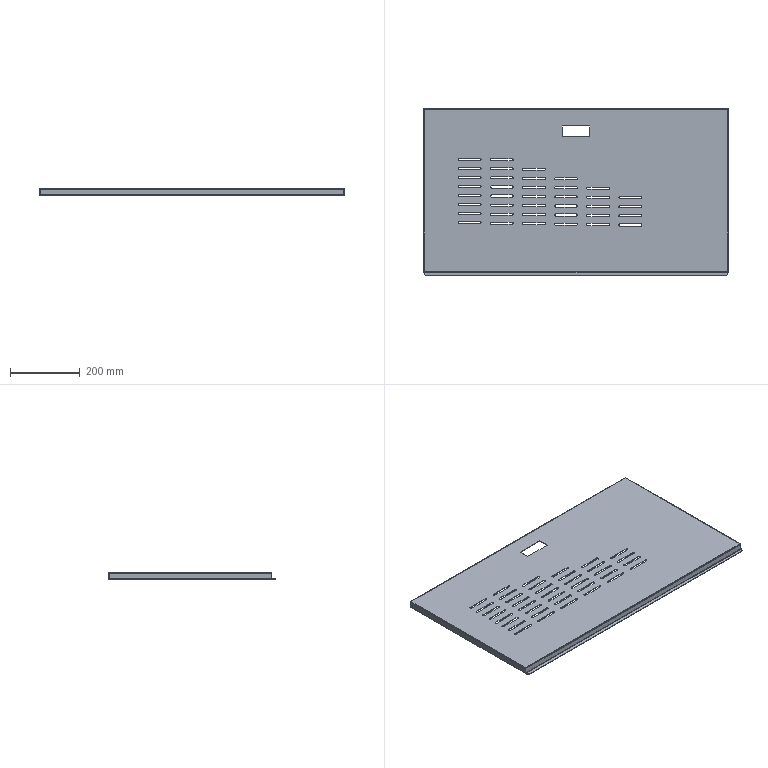Part | STEP file | Electrical Cabinet Lower Box Closing Plate | 1 solid | 278 faces | box 876 x 479.5 x 19.5 mm | volume 704453 mm3 | plane 134 | cylinder 132 | spline 12 | commonest cylinder face diameters 6 x114 1 x8 4 x8 20 x2